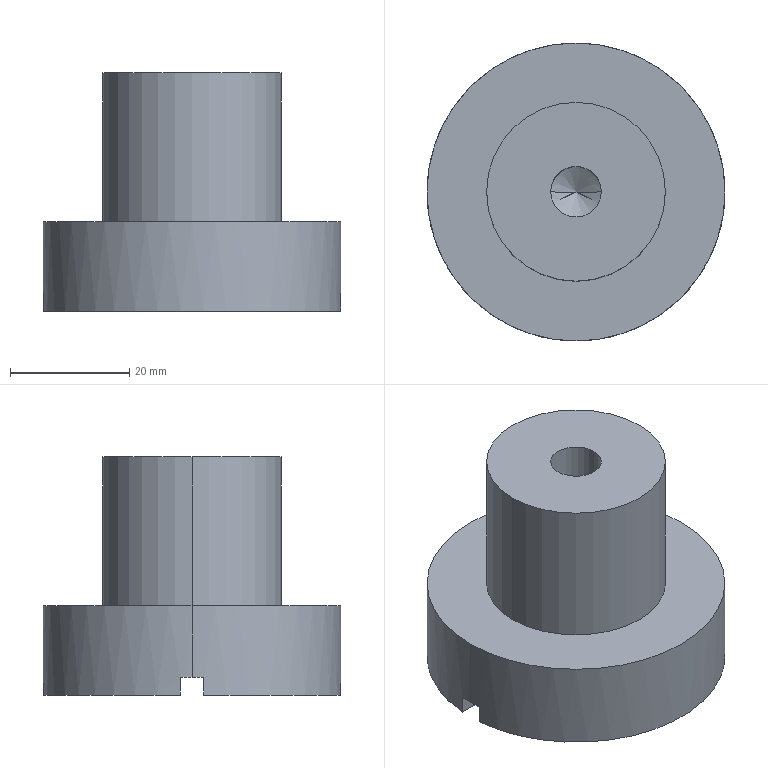Part | STEP file | Knob QY-1-20 | 1 solid | 15 faces | box 50 x 50 x 40 mm | volume 45086 mm3 | plane 7 | cylinder 6 | cone 2 | commonest cylinder face diameters 8.5 x2 30 x2 50 x2
STEP:
#1=CARTESIAN_POINT('',(0.,0.,0.));
#2=DIRECTION('',(0.,0.,1.));
#3=DIRECTION('',(1.,0.,0.));
#4=AXIS2_PLACEMENT_3D('',#1,#2,#3);
#5=CARTESIAN_POINT('',(4.25,0.,15.5));
#6=VERTEX_POINT('',#5);
#7=CARTESIAN_POINT('',(4.25,0.,40.));
#8=VERTEX_POINT('',#7);
#9=CARTESIAN_POINT('',(4.25,0.,40.));
#10=DIRECTION('',(0.,0.,1.));
#11=VECTOR('',#10,1.);
#12=LINE('',#9,#11);
#13=CARTESIAN_POINT('',(0.,0.,40.));
#14=DIRECTION('',(0.,0.,1.));
#15=DIRECTION('',(1.,0.,0.));
#16=AXIS2_PLACEMENT_3D('',#13,#14,#15);
#17=CYLINDRICAL_SURFACE('',#16,4.25);
#18=CARTESIAN_POINT('',(6.283,0.));
#19=DIRECTION('',(0.,1.));
#20=VECTOR('',#19,1.);
#21=LINE('',#18,#20);
#22=(GEOMETRIC_REPRESENTATION_CONTEXT(2)PARAMETRIC_REPRESENTATION_CONTEXT()REPRESENTATION_CONTEXT('',''));
#23=DEFINITIONAL_REPRESENTATION('',(#21),#22);
#24=PCURVE('',#17,#23);
#25=CARTESIAN_POINT('',(0.,0.,40.));
#26=DIRECTION('',(0.,0.,1.));
#27=DIRECTION('',(1.,0.,0.));
#28=AXIS2_PLACEMENT_3D('',#25,#26,#27);
#29=CYLINDRICAL_SURFACE('',#28,4.25);
#30=CARTESIAN_POINT('',(0.,0.));
#31=DIRECTION('',(0.,1.));
#32=VECTOR('',#31,1.);
#33=LINE('',#30,#32);
#34=(GEOMETRIC_REPRESENTATION_CONTEXT(2)PARAMETRIC_REPRESENTATION_CONTEXT()REPRESENTATION_CONTEXT('',''));
#35=DEFINITIONAL_REPRESENTATION('',(#33),#34);
#36=PCURVE('',#29,#35);
#37=SURFACE_CURVE('',#12,(#24,#36),.PCURVE_S1.);
#38=EDGE_CURVE('',#6,#8,#37,.T.);
#39=ORIENTED_EDGE('',*,*,#38,.T.);
#40=CARTESIAN_POINT('',(-4.25,0.,40.));
#41=VERTEX_POINT('',#40);
#42=CARTESIAN_POINT('',(0.,0.,40.));
#43=DIRECTION('',(0.,0.,1.));
#44=DIRECTION('',(1.,0.,0.));
#45=AXIS2_PLACEMENT_3D('',#42,#43,#44);
#46=CIRCLE('',#45,4.25);
#47=CARTESIAN_POINT('',(0.,0.));
#48=DIRECTION('',(1.,0.));
#49=VECTOR('',#48,1.);
#50=LINE('',#47,#49);
#51=(GEOMETRIC_REPRESENTATION_CONTEXT(2)PARAMETRIC_REPRESENTATION_CONTEXT()REPRESENTATION_CONTEXT('',''));
#52=DEFINITIONAL_REPRESENTATION('',(#50),#51);
#53=PCURVE('',#17,#52);
#54=CARTESIAN_POINT('',(0.,0.,40.));
#55=DIRECTION('',(0.,0.,1.));
#56=DIRECTION('',(1.,0.,0.));
#57=AXIS2_PLACEMENT_3D('',#54,#55,#56);
#58=PLANE('',#57);
#59=CARTESIAN_POINT('',(0.,0.));
#60=DIRECTION('',(1.,0.));
#61=AXIS2_PLACEMENT_2D('',#59,#60);
#62=CIRCLE('',#61,4.25);
#63=(GEOMETRIC_REPRESENTATION_CONTEXT(2)PARAMETRIC_REPRESENTATION_CONTEXT()REPRESENTATION_CONTEXT('',''));
#64=DEFINITIONAL_REPRESENTATION('',(#62),#63);
#65=PCURVE('',#58,#64);
#66=SURFACE_CURVE('',#46,(#53,#65),.PCURVE_S1.);
#67=EDGE_CURVE('',#41,#8,#66,.T.);
#68=ORIENTED_EDGE('',*,*,#67,.F.);
#69=CARTESIAN_POINT('',(-4.25,0.,15.5));
#70=VERTEX_POINT('',#69);
#71=CARTESIAN_POINT('',(-4.25,0.,40.));
#72=DIRECTION('',(0.,0.,1.));
#73=VECTOR('',#72,1.);
#74=LINE('',#71,#73);
#75=CARTESIAN_POINT('',(3.142,0.));
#76=DIRECTION('',(0.,1.));
#77=VECTOR('',#76,1.);
#78=LINE('',#75,#77);
#79=(GEOMETRIC_REPRESENTATION_CONTEXT(2)PARAMETRIC_REPRESENTATION_CONTEXT()REPRESENTATION_CONTEXT('',''));
#80=DEFINITIONAL_REPRESENTATION('',(#78),#79);
#81=PCURVE('',#17,#80);
#82=CARTESIAN_POINT('',(3.142,0.));
#83=DIRECTION('',(0.,1.));
#84=VECTOR('',#83,1.);
#85=LINE('',#82,#84);
#86=(GEOMETRIC_REPRESENTATION_CONTEXT(2)PARAMETRIC_REPRESENTATION_CONTEXT()REPRESENTATION_CONTEXT('',''));
#87=DEFINITIONAL_REPRESENTATION('',(#85),#86);
#88=PCURVE('',#29,#87);
#89=SURFACE_CURVE('',#74,(#81,#88),.PCURVE_S1.);
#90=EDGE_CURVE('',#70,#41,#89,.T.);
#91=ORIENTED_EDGE('',*,*,#90,.F.);
#92=CARTESIAN_POINT('',(0.,0.,15.5));
#93=DIRECTION('',(0.,0.,1.));
#94=DIRECTION('',(1.,0.,0.));
#95=AXIS2_PLACEMENT_3D('',#92,#93,#94);
#96=CIRCLE('',#95,4.25);
#97=CARTESIAN_POINT('',(0.,-24.5));
#98=DIRECTION('',(1.,0.));
#99=VECTOR('',#98,1.);
#100=LINE('',#97,#99);
#101=(GEOMETRIC_REPRESENTATION_CONTEXT(2)PARAMETRIC_REPRESENTATION_CONTEXT()REPRESENTATION_CONTEXT('',''));
#102=DEFINITIONAL_REPRESENTATION('',(#100),#101);
#103=PCURVE('',#17,#102);
#104=CARTESIAN_POINT('',(0.,0.,15.5));
#105=DIRECTION('',(0.,0.,1.));
#106=DIRECTION('',(1.,0.,0.));
#107=AXIS2_PLACEMENT_3D('',#104,#105,#106);
#108=CONICAL_SURFACE('',#107,4.25,1.03);
#109=CARTESIAN_POINT('',(0.,0.));
#110=DIRECTION('',(1.,0.));
#111=VECTOR('',#110,1.);
#112=LINE('',#109,#111);
#113=(GEOMETRIC_REPRESENTATION_CONTEXT(2)PARAMETRIC_REPRESENTATION_CONTEXT()REPRESENTATION_CONTEXT('',''));
#114=DEFINITIONAL_REPRESENTATION('',(#112),#113);
#115=PCURVE('',#108,#114);
#116=SURFACE_CURVE('',#96,(#103,#115),.PCURVE_S1.);
#117=EDGE_CURVE('',#70,#6,#116,.T.);
#118=ORIENTED_EDGE('',*,*,#117,.T.);
#119=EDGE_LOOP('',(#39,#68,#91,#118));
#120=FACE_BOUND('',#119,.F.);
#121=ADVANCED_FACE('',(#120),#17,.F.);
#122=ORIENTED_EDGE('',*,*,#117,.F.);
#123=CARTESIAN_POINT('',(0.,0.,12.946));
#124=VERTEX_POINT('',#123);
#125=CARTESIAN_POINT('',(-4.25,0.,15.5));
#126=DIRECTION('',(-0.8572,0.,0.515));
#127=VECTOR('',#126,1.);
#128=LINE('',#125,#127);
#129=CARTESIAN_POINT('',(3.142,0.));
#130=DIRECTION('',(0.,1.));
#131=VECTOR('',#130,1.);
#132=LINE('',#129,#131);
#133=(GEOMETRIC_REPRESENTATION_CONTEXT(2)PARAMETRIC_REPRESENTATION_CONTEXT()REPRESENTATION_CONTEXT('',''));
#134=DEFINITIONAL_REPRESENTATION('',(#132),#133);
#135=PCURVE('',#108,#134);
#136=CARTESIAN_POINT('',(0.,0.,15.5));
#137=DIRECTION('',(0.,0.,1.));
#138=DIRECTION('',(1.,0.,0.));
#139=AXIS2_PLACEMENT_3D('',#136,#137,#138);
#140=CONICAL_SURFACE('',#139,4.25,1.03);
#141=CARTESIAN_POINT('',(3.142,0.));
#142=DIRECTION('',(0.,1.));
#143=VECTOR('',#142,1.);
#144=LINE('',#141,#143);
#145=(GEOMETRIC_REPRESENTATION_CONTEXT(2)PARAMETRIC_REPRESENTATION_CONTEXT()REPRESENTATION_CONTEXT('',''));
#146=DEFINITIONAL_REPRESENTATION('',(#144),#145);
#147=PCURVE('',#140,#146);
#148=SURFACE_CURVE('',#128,(#135,#147),.PCURVE_S1.);
#149=EDGE_CURVE('',#124,#70,#148,.T.);
#150=ORIENTED_EDGE('',*,*,#149,.F.);
#151=CARTESIAN_POINT('',(4.25,0.,15.5));
#152=DIRECTION('',(0.8572,0.,0.515));
#153=VECTOR('',#152,1.);
#154=LINE('',#151,#153);
#155=CARTESIAN_POINT('',(6.283,0.));
#156=DIRECTION('',(0.,1.));
#157=VECTOR('',#156,1.);
#158=LINE('',#155,#157);
#159=(GEOMETRIC_REPRESENTATION_CONTEXT(2)PARAMETRIC_REPRESENTATION_CONTEXT()REPRESENTATION_CONTEXT('',''));
#160=DEFINITIONAL_REPRESENTATION('',(#158),#159);
#161=PCURVE('',#108,#160);
#162=CARTESIAN_POINT('',(0.,0.));
#163=DIRECTION('',(0.,1.));
#164=VECTOR('',#163,1.);
#165=LINE('',#162,#164);
#166=(GEOMETRIC_REPRESENTATION_CONTEXT(2)PARAMETRIC_REPRESENTATION_CONTEXT()REPRESENTATION_CONTEXT('',''));
#167=DEFINITIONAL_REPRESENTATION('',(#165),#166);
#168=PCURVE('',#140,#167);
#169=SURFACE_CURVE('',#154,(#161,#168),.PCURVE_S1.);
#170=EDGE_CURVE('',#124,#6,#169,.T.);
#171=ORIENTED_EDGE('',*,*,#170,.T.);
#172=EDGE_LOOP('',(#122,#150,#171));
#173=FACE_BOUND('',#172,.F.);
#174=ADVANCED_FACE('',(#173),#108,.F.);
#175=CARTESIAN_POINT('',(15.,0.,40.));
#176=VERTEX_POINT('',#175);
#177=CARTESIAN_POINT('',(-15.,0.,40.));
#178=VERTEX_POINT('',#177);
#179=CARTESIAN_POINT('',(0.,0.,40.));
#180=DIRECTION('',(0.,0.,1.));
#181=DIRECTION('',(1.,0.,0.));
#182=AXIS2_PLACEMENT_3D('',#179,#180,#181);
#183=CIRCLE('',#182,15.);
#184=CARTESIAN_POINT('',(0.,0.,40.));
#185=DIRECTION('',(0.,0.,-1.));
#186=DIRECTION('',(-1.,0.,0.));
#187=AXIS2_PLACEMENT_3D('',#184,#185,#186);
#188=CYLINDRICAL_SURFACE('',#187,15.);
#189=CARTESIAN_POINT('',(3.142,0.));
#190=DIRECTION('',(-1.,0.));
#191=VECTOR('',#190,1.);
#192=LINE('',#189,#191);
#193=(GEOMETRIC_REPRESENTATION_CONTEXT(2)PARAMETRIC_REPRESENTATION_CONTEXT()REPRESENTATION_CONTEXT('',''));
#194=DEFINITIONAL_REPRESENTATION('',(#192),#193);
#195=PCURVE('',#188,#194);
#196=CARTESIAN_POINT('',(0.,0.));
#197=DIRECTION('',(1.,0.));
#198=AXIS2_PLACEMENT_2D('',#196,#197);
#199=CIRCLE('',#198,15.);
#200=(GEOMETRIC_REPRESENTATION_CONTEXT(2)PARAMETRIC_REPRESENTATION_CONTEXT()REPRESENTATION_CONTEXT('',''));
#201=DEFINITIONAL_REPRESENTATION('',(#199),#200);
#202=PCURVE('',#58,#201);
#203=SURFACE_CURVE('',#183,(#195,#202),.PCURVE_S1.);
#204=EDGE_CURVE('',#176,#178,#203,.T.);
#205=ORIENTED_EDGE('',*,*,#204,.F.);
#206=CARTESIAN_POINT('',(15.,0.,15.));
#207=VERTEX_POINT('',#206);
#208=CARTESIAN_POINT('',(15.,0.,40.));
#209=DIRECTION('',(0.,0.,-1.));
#210=VECTOR('',#209,1.);
#211=LINE('',#208,#210);
#212=CARTESIAN_POINT('',(3.142,0.));
#213=DIRECTION('',(0.,1.));
#214=VECTOR('',#213,1.);
#215=LINE('',#212,#214);
#216=(GEOMETRIC_REPRESENTATION_CONTEXT(2)PARAMETRIC_REPRESENTATION_CONTEXT()REPRESENTATION_CONTEXT('',''));
#217=DEFINITIONAL_REPRESENTATION('',(#215),#216);
#218=PCURVE('',#188,#217);
#219=CARTESIAN_POINT('',(0.,0.,40.));
#220=DIRECTION('',(0.,0.,-1.));
#221=DIRECTION('',(-1.,0.,0.));
#222=AXIS2_PLACEMENT_3D('',#219,#220,#221);
#223=CYLINDRICAL_SURFACE('',#222,15.);
#224=CARTESIAN_POINT('',(3.142,0.));
#225=DIRECTION('',(0.,1.));
#226=VECTOR('',#225,1.);
#227=LINE('',#224,#226);
#228=(GEOMETRIC_REPRESENTATION_CONTEXT(2)PARAMETRIC_REPRESENTATION_CONTEXT()REPRESENTATION_CONTEXT('',''));
#229=DEFINITIONAL_REPRESENTATION('',(#227),#228);
#230=PCURVE('',#223,#229);
#231=SURFACE_CURVE('',#211,(#218,#230),.PCURVE_S1.);
#232=EDGE_CURVE('',#176,#207,#231,.T.);
#233=ORIENTED_EDGE('',*,*,#232,.T.);
#234=CARTESIAN_POINT('',(-15.,0.,15.));
#235=VERTEX_POINT('',#234);
#236=CARTESIAN_POINT('',(0.,0.,15.));
#237=DIRECTION('',(0.,0.,1.));
#238=DIRECTION('',(1.,0.,0.));
#239=AXIS2_PLACEMENT_3D('',#236,#237,#238);
#240=CIRCLE('',#239,15.);
#241=CARTESIAN_POINT('',(3.142,25.));
#242=DIRECTION('',(-1.,0.));
#243=VECTOR('',#242,1.);
#244=LINE('',#241,#243);
#245=(GEOMETRIC_REPRESENTATION_CONTEXT(2)PARAMETRIC_REPRESENTATION_CONTEXT()REPRESENTATION_CONTEXT('',''));
#246=DEFINITIONAL_REPRESENTATION('',(#244),#245);
#247=PCURVE('',#188,#246);
#248=CARTESIAN_POINT('',(0.,0.,15.));
#249=DIRECTION('',(0.,0.,1.));
#250=DIRECTION('',(1.,0.,0.));
#251=AXIS2_PLACEMENT_3D('',#248,#249,#250);
#252=PLANE('',#251);
#253=CARTESIAN_POINT('',(0.,0.));
#254=DIRECTION('',(1.,0.));
#255=AXIS2_PLACEMENT_2D('',#253,#254);
#256=CIRCLE('',#255,15.);
#257=(GEOMETRIC_REPRESENTATION_CONTEXT(2)PARAMETRIC_REPRESENTATION_CONTEXT()REPRESENTATION_CONTEXT('',''));
#258=DEFINITIONAL_REPRESENTATION('',(#256),#257);
#259=PCURVE('',#252,#258);
#260=SURFACE_CURVE('',#240,(#247,#259),.PCURVE_S1.);
#261=EDGE_CURVE('',#207,#235,#260,.T.);
#262=ORIENTED_EDGE('',*,*,#261,.T.);
#263=CARTESIAN_POINT('',(-15.,0.,40.));
#264=DIRECTION('',(0.,0.,-1.));
#265=VECTOR('',#264,1.);
#266=LINE('',#263,#265);
#267=CARTESIAN_POINT('',(0.,0.));
#268=DIRECTION('',(0.,1.));
#269=VECTOR('',#268,1.);
#270=LINE('',#267,#269);
#271=(GEOMETRIC_REPRESENTATION_CONTEXT(2)PARAMETRIC_REPRESENTATION_CONTEXT()REPRESENTATION_CONTEXT('',''));
#272=DEFINITIONAL_REPRESENTATION('',(#270),#271);
#273=PCURVE('',#188,#272);
#274=CARTESIAN_POINT('',(6.283,0.));
#275=DIRECTION('',(0.,1.));
#276=VECTOR('',#275,1.);
#277=LINE('',#274,#276);
#278=(GEOMETRIC_REPRESENTATION_CONTEXT(2)PARAMETRIC_REPRESENTATION_CONTEXT()REPRESENTATION_CONTEXT('',''));
#279=DEFINITIONAL_REPRESENTATION('',(#277),#278);
#280=PCURVE('',#223,#279);
#281=SURFACE_CURVE('',#266,(#273,#280),.PCURVE_S1.);
#282=EDGE_CURVE('',#178,#235,#281,.T.);
#283=ORIENTED_EDGE('',*,*,#282,.F.);
#284=EDGE_LOOP('',(#205,#233,#262,#283));
#285=FACE_BOUND('',#284,.T.);
#286=ADVANCED_FACE('',(#285),#188,.T.);
#287=CARTESIAN_POINT('',(25.,0.,15.));
#288=VERTEX_POINT('',#287);
#289=CARTESIAN_POINT('',(-25.,0.,15.));
#290=VERTEX_POINT('',#289);
#291=CARTESIAN_POINT('',(0.,0.,15.));
#292=DIRECTION('',(0.,0.,1.));
#293=DIRECTION('',(1.,0.,0.));
#294=AXIS2_PLACEMENT_3D('',#291,#292,#293);
#295=CIRCLE('',#294,25.);
#296=CARTESIAN_POINT('',(0.,0.,15.));
#297=DIRECTION('',(0.,0.,-1.));
#298=DIRECTION('',(-1.,0.,0.));
#299=AXIS2_PLACEMENT_3D('',#296,#297,#298);
#300=CYLINDRICAL_SURFACE('',#299,25.);
#301=CARTESIAN_POINT('',(3.142,0.));
#302=DIRECTION('',(-1.,0.));
#303=VECTOR('',#302,1.);
#304=LINE('',#301,#303);
#305=(GEOMETRIC_REPRESENTATION_CONTEXT(2)PARAMETRIC_REPRESENTATION_CONTEXT()REPRESENTATION_CONTEXT('',''));
#306=DEFINITIONAL_REPRESENTATION('',(#304),#305);
#307=PCURVE('',#300,#306);
#308=CARTESIAN_POINT('',(0.,0.));
#309=DIRECTION('',(1.,0.));
#310=AXIS2_PLACEMENT_2D('',#308,#309);
#311=CIRCLE('',#310,25.);
#312=(GEOMETRIC_REPRESENTATION_CONTEXT(2)PARAMETRIC_REPRESENTATION_CONTEXT()REPRESENTATION_CONTEXT('',''));
#313=DEFINITIONAL_REPRESENTATION('',(#311),#312);
#314=PCURVE('',#252,#313);
#315=SURFACE_CURVE('',#295,(#307,#314),.PCURVE_S1.);
#316=EDGE_CURVE('',#288,#290,#315,.T.);
#317=ORIENTED_EDGE('',*,*,#316,.F.);
#318=CARTESIAN_POINT('',(25.,0.,3.));
#319=VERTEX_POINT('',#318);
#320=CARTESIAN_POINT('',(25.,0.,15.));
#321=DIRECTION('',(0.,0.,-1.));
#322=VECTOR('',#321,1.);
#323=LINE('',#320,#322);
#324=CARTESIAN_POINT('',(3.142,0.));
#325=DIRECTION('',(0.,1.));
#326=VECTOR('',#325,1.);
#327=LINE('',#324,#326);
#328=(GEOMETRIC_REPRESENTATION_CONTEXT(2)PARAMETRIC_REPRESENTATION_CONTEXT()REPRESENTATION_CONTEXT('',''));
#329=DEFINITIONAL_REPRESENTATION('',(#327),#328);
#330=PCURVE('',#300,#329);
#331=CARTESIAN_POINT('',(0.,0.,15.));
#332=DIRECTION('',(0.,0.,-1.));
#333=DIRECTION('',(-1.,0.,0.));
#334=AXIS2_PLACEMENT_3D('',#331,#332,#333);
#335=CYLINDRICAL_SURFACE('',#334,25.);
#336=CARTESIAN_POINT('',(3.142,0.));
#337=DIRECTION('',(0.,1.));
#338=VECTOR('',#337,1.);
#339=LINE('',#336,#338);
#340=(GEOMETRIC_REPRESENTATION_CONTEXT(2)PARAMETRIC_REPRESENTATION_CONTEXT()REPRESENTATION_CONTEXT('',''));
#341=DEFINITIONAL_REPRESENTATION('',(#339),#340);
#342=PCURVE('',#335,#341);
#343=SURFACE_CURVE('',#323,(#330,#342),.PCURVE_S1.);
#344=EDGE_CURVE('',#288,#319,#343,.T.);
#345=ORIENTED_EDGE('',*,*,#344,.T.);
#346=CARTESIAN_POINT('',(24.92,2.,3.));
#347=VERTEX_POINT('',#346);
#348=CARTESIAN_POINT('',(0.,0.,3.));
#349=DIRECTION('',(0.,0.,-1.));
#350=DIRECTION('',(-1.,0.,0.));
#351=AXIS2_PLACEMENT_3D('',#348,#349,#350);
#352=CIRCLE('',#351,25.);
#353=CARTESIAN_POINT('',(0.,12.));
#354=DIRECTION('',(1.,0.));
#355=VECTOR('',#354,1.);
#356=LINE('',#353,#355);
#357=(GEOMETRIC_REPRESENTATION_CONTEXT(2)PARAMETRIC_REPRESENTATION_CONTEXT()REPRESENTATION_CONTEXT('',''));
#358=DEFINITIONAL_REPRESENTATION('',(#356),#357);
#359=PCURVE('',#300,#358);
#360=CARTESIAN_POINT('',(0.,0.,3.));
#361=DIRECTION('',(0.,0.,-1.));
#362=DIRECTION('',(-1.,0.,0.));
#363=AXIS2_PLACEMENT_3D('',#360,#361,#362);
#364=PLANE('',#363);
#365=CARTESIAN_POINT('',(0.,0.));
#366=DIRECTION('',(1.,0.));
#367=AXIS2_PLACEMENT_2D('',#365,#366);
#368=CIRCLE('',#367,25.);
#369=(GEOMETRIC_REPRESENTATION_CONTEXT(2)PARAMETRIC_REPRESENTATION_CONTEXT()REPRESENTATION_CONTEXT('',''));
#370=DEFINITIONAL_REPRESENTATION('',(#368),#369);
#371=PCURVE('',#364,#370);
#372=SURFACE_CURVE('',#352,(#359,#371),.PCURVE_S1.);
#373=EDGE_CURVE('',#347,#319,#372,.T.);
#374=ORIENTED_EDGE('',*,*,#373,.F.);
#375=CARTESIAN_POINT('',(24.92,2.,0.));
#376=VERTEX_POINT('',#375);
#377=CARTESIAN_POINT('',(24.92,2.,15.));
#378=DIRECTION('',(0.,0.,-1.));
#379=VECTOR('',#378,1.);
#380=LINE('',#377,#379);
#381=CARTESIAN_POINT('',(3.062,0.));
#382=DIRECTION('',(0.,1.));
#383=VECTOR('',#382,1.);
#384=LINE('',#381,#383);
#385=(GEOMETRIC_REPRESENTATION_CONTEXT(2)PARAMETRIC_REPRESENTATION_CONTEXT()REPRESENTATION_CONTEXT('',''));
#386=DEFINITIONAL_REPRESENTATION('',(#384),#385);
#387=PCURVE('',#300,#386);
#388=CARTESIAN_POINT('',(34.879,2.,3.));
#389=DIRECTION('',(0.,1.,0.));
#390=DIRECTION('',(0.,0.,1.));
#391=AXIS2_PLACEMENT_3D('',#388,#389,#390);
#392=PLANE('',#391);
#393=CARTESIAN_POINT('',(12.,-9.959));
#394=DIRECTION('',(-1.,0.));
#395=VECTOR('',#394,1.);
#396=LINE('',#393,#395);
#397=(GEOMETRIC_REPRESENTATION_CONTEXT(2)PARAMETRIC_REPRESENTATION_CONTEXT()REPRESENTATION_CONTEXT('',''));
#398=DEFINITIONAL_REPRESENTATION('',(#396),#397);
#399=PCURVE('',#392,#398);
#400=SURFACE_CURVE('',#380,(#387,#399),.PCURVE_S1.);
#401=EDGE_CURVE('',#347,#376,#400,.T.);
#402=ORIENTED_EDGE('',*,*,#401,.T.);
#403=CARTESIAN_POINT('',(-24.92,2.,0.));
#404=VERTEX_POINT('',#403);
#405=CARTESIAN_POINT('',(0.,0.,0.));
#406=DIRECTION('',(0.,0.,1.));
#407=DIRECTION('',(1.,0.,0.));
#408=AXIS2_PLACEMENT_3D('',#405,#406,#407);
#409=CIRCLE('',#408,25.);
#410=CARTESIAN_POINT('',(3.142,15.));
#411=DIRECTION('',(-1.,0.));
#412=VECTOR('',#411,1.);
#413=LINE('',#410,#412);
#414=(GEOMETRIC_REPRESENTATION_CONTEXT(2)PARAMETRIC_REPRESENTATION_CONTEXT()REPRESENTATION_CONTEXT('',''));
#415=DEFINITIONAL_REPRESENTATION('',(#413),#414);
#416=PCURVE('',#300,#415);
#417=CARTESIAN_POINT('',(0.,0.,0.));
#418=DIRECTION('',(0.,0.,1.));
#419=DIRECTION('',(1.,0.,0.));
#420=AXIS2_PLACEMENT_3D('',#417,#418,#419);
#421=PLANE('',#420);
#422=CARTESIAN_POINT('',(0.,0.));
#423=DIRECTION('',(1.,0.));
#424=AXIS2_PLACEMENT_2D('',#422,#423);
#425=CIRCLE('',#424,25.);
#426=(GEOMETRIC_REPRESENTATION_CONTEXT(2)PARAMETRIC_REPRESENTATION_CONTEXT()REPRESENTATION_CONTEXT('',''));
#427=DEFINITIONAL_REPRESENTATION('',(#425),#426);
#428=PCURVE('',#421,#427);
#429=SURFACE_CURVE('',#409,(#416,#428),.PCURVE_S1.);
#430=EDGE_CURVE('',#376,#404,#429,.T.);
#431=ORIENTED_EDGE('',*,*,#430,.T.);
#432=CARTESIAN_POINT('',(-24.92,2.,3.));
#433=VERTEX_POINT('',#432);
#434=CARTESIAN_POINT('',(-24.92,2.,15.));
#435=DIRECTION('',(0.,0.,1.));
#436=VECTOR('',#435,1.);
#437=LINE('',#434,#436);
#438=CARTESIAN_POINT('',(0.08009,0.));
#439=DIRECTION('',(0.,-1.));
#440=VECTOR('',#439,1.);
#441=LINE('',#438,#440);
#442=(GEOMETRIC_REPRESENTATION_CONTEXT(2)PARAMETRIC_REPRESENTATION_CONTEXT()REPRESENTATION_CONTEXT('',''));
#443=DEFINITIONAL_REPRESENTATION('',(#441),#442);
#444=PCURVE('',#300,#443);
#445=CARTESIAN_POINT('',(12.,-59.799));
#446=DIRECTION('',(1.,0.));
#447=VECTOR('',#446,1.);
#448=LINE('',#445,#447);
#449=(GEOMETRIC_REPRESENTATION_CONTEXT(2)PARAMETRIC_REPRESENTATION_CONTEXT()REPRESENTATION_CONTEXT('',''));
#450=DEFINITIONAL_REPRESENTATION('',(#448),#449);
#451=PCURVE('',#392,#450);
#452=SURFACE_CURVE('',#437,(#444,#451),.PCURVE_S1.);
#453=EDGE_CURVE('',#404,#433,#452,.T.);
#454=ORIENTED_EDGE('',*,*,#453,.T.);
#455=CARTESIAN_POINT('',(-25.,0.,3.));
#456=VERTEX_POINT('',#455);
#457=CARTESIAN_POINT('',(0.,0.,3.));
#458=DIRECTION('',(0.,0.,-1.));
#459=DIRECTION('',(-1.,0.,0.));
#460=AXIS2_PLACEMENT_3D('',#457,#458,#459);
#461=CIRCLE('',#460,25.);
#462=CARTESIAN_POINT('',(0.,12.));
#463=DIRECTION('',(1.,0.));
#464=VECTOR('',#463,1.);
#465=LINE('',#462,#464);
#466=(GEOMETRIC_REPRESENTATION_CONTEXT(2)PARAMETRIC_REPRESENTATION_CONTEXT()REPRESENTATION_CONTEXT('',''));
#467=DEFINITIONAL_REPRESENTATION('',(#465),#466);
#468=PCURVE('',#300,#467);
#469=CARTESIAN_POINT('',(0.,0.));
#470=DIRECTION('',(1.,0.));
#471=AXIS2_PLACEMENT_2D('',#469,#470);
#472=CIRCLE('',#471,25.);
#473=(GEOMETRIC_REPRESENTATION_CONTEXT(2)PARAMETRIC_REPRESENTATION_CONTEXT()REPRESENTATION_CONTEXT('',''));
#474=DEFINITIONAL_REPRESENTATION('',(#472),#473);
#475=PCURVE('',#364,#474);
#476=SURFACE_CURVE('',#461,(#468,#475),.PCURVE_S1.);
#477=EDGE_CURVE('',#456,#433,#476,.T.);
#478=ORIENTED_EDGE('',*,*,#477,.F.);
#479=CARTESIAN_POINT('',(-25.,0.,15.));
#480=DIRECTION('',(0.,0.,-1.));
#481=VECTOR('',#480,1.);
#482=LINE('',#479,#481);
#483=CARTESIAN_POINT('',(0.,0.));
#484=DIRECTION('',(0.,1.));
#485=VECTOR('',#484,1.);
#486=LINE('',#483,#485);
#487=(GEOMETRIC_REPRESENTATION_CONTEXT(2)PARAMETRIC_REPRESENTATION_CONTEXT()REPRESENTATION_CONTEXT('',''));
#488=DEFINITIONAL_REPRESENTATION('',(#486),#487);
#489=PCURVE('',#300,#488);
#490=CARTESIAN_POINT('',(6.283,0.));
#491=DIRECTION('',(0.,1.));
#492=VECTOR('',#491,1.);
#493=LINE('',#490,#492);
#494=(GEOMETRIC_REPRESENTATION_CONTEXT(2)PARAMETRIC_REPRESENTATION_CONTEXT()REPRESENTATION_CONTEXT('',''));
#495=DEFINITIONAL_REPRESENTATION('',(#493),#494);
#496=PCURVE('',#335,#495);
#497=SURFACE_CURVE('',#482,(#489,#496),.PCURVE_S1.);
#498=EDGE_CURVE('',#290,#456,#497,.T.);
#499=ORIENTED_EDGE('',*,*,#498,.F.);
#500=EDGE_LOOP('',(#317,#345,#374,#402,#431,#454,#478,#499));
#501=FACE_BOUND('',#500,.T.);
#502=ADVANCED_FACE('',(#501),#300,.T.);
#503=CARTESIAN_POINT('',(-24.92,-2.,0.));
#504=VERTEX_POINT('',#503);
#505=CARTESIAN_POINT('',(24.92,-2.,0.));
#506=VERTEX_POINT('',#505);
#507=CARTESIAN_POINT('',(0.,0.,0.));
#508=DIRECTION('',(0.,0.,1.));
#509=DIRECTION('',(1.,0.,0.));
#510=AXIS2_PLACEMENT_3D('',#507,#508,#509);
#511=CIRCLE('',#510,25.);
#512=CARTESIAN_POINT('',(0.,0.,0.));
#513=DIRECTION('',(0.,0.,1.));
#514=DIRECTION('',(1.,0.,0.));
#515=AXIS2_PLACEMENT_3D('',#512,#513,#514);
#516=PLANE('',#515);
#517=CARTESIAN_POINT('',(0.,0.));
#518=DIRECTION('',(1.,0.));
#519=AXIS2_PLACEMENT_2D('',#517,#518);
#520=CIRCLE('',#519,25.);
#521=(GEOMETRIC_REPRESENTATION_CONTEXT(2)PARAMETRIC_REPRESENTATION_CONTEXT()REPRESENTATION_CONTEXT('',''));
#522=DEFINITIONAL_REPRESENTATION('',(#520),#521);
#523=PCURVE('',#516,#522);
#524=CARTESIAN_POINT('',(9.425,15.));
#525=DIRECTION('',(-1.,0.));
#526=VECTOR('',#525,1.);
#527=LINE('',#524,#526);
#528=(GEOMETRIC_REPRESENTATION_CONTEXT(2)PARAMETRIC_REPRESENTATION_CONTEXT()REPRESENTATION_CONTEXT('',''));
#529=DEFINITIONAL_REPRESENTATION('',(#527),#528);
#530=PCURVE('',#335,#529);
#531=SURFACE_CURVE('',#511,(#523,#530),.PCURVE_S1.);
#532=EDGE_CURVE('',#504,#506,#531,.T.);
#533=ORIENTED_EDGE('',*,*,#532,.F.);
#534=CARTESIAN_POINT('',(0.,-2.,0.));
#535=DIRECTION('',(1.,0.,0.));
#536=VECTOR('',#535,1.);
#537=LINE('',#534,#536);
#538=CARTESIAN_POINT('',(0.,-2.));
#539=DIRECTION('',(1.,0.));
#540=VECTOR('',#539,1.);
#541=LINE('',#538,#540);
#542=(GEOMETRIC_REPRESENTATION_CONTEXT(2)PARAMETRIC_REPRESENTATION_CONTEXT()REPRESENTATION_CONTEXT('',''));
#543=DEFINITIONAL_REPRESENTATION('',(#541),#542);
#544=PCURVE('',#516,#543);
#545=CARTESIAN_POINT('',(34.879,-2.,3.));
#546=DIRECTION('',(0.,-1.,0.));
#547=DIRECTION('',(0.,0.,-1.));
#548=AXIS2_PLACEMENT_3D('',#545,#546,#547);
#549=PLANE('',#548);
#550=CARTESIAN_POINT('',(3.,-34.879));
#551=DIRECTION('',(0.,1.));
#552=VECTOR('',#551,1.);
#553=LINE('',#550,#552);
#554=(GEOMETRIC_REPRESENTATION_CONTEXT(2)PARAMETRIC_REPRESENTATION_CONTEXT()REPRESENTATION_CONTEXT('',''));
#555=DEFINITIONAL_REPRESENTATION('',(#553),#554);
#556=PCURVE('',#549,#555);
#557=SURFACE_CURVE('',#537,(#544,#556),.PCURVE_S1.);
#558=EDGE_CURVE('',#504,#506,#557,.T.);
#559=ORIENTED_EDGE('',*,*,#558,.T.);
#560=EDGE_LOOP('',(#533,#559));
#561=FACE_BOUND('',#560,.T.);
#562=ADVANCED_FACE('',(#561),#516,.F.);
#563=ORIENTED_EDGE('',*,*,#344,.F.);
#564=CARTESIAN_POINT('',(0.,0.,15.));
#565=DIRECTION('',(0.,0.,1.));
#566=DIRECTION('',(1.,0.,0.));
#567=AXIS2_PLACEMENT_3D('',#564,#565,#566);
#568=CIRCLE('',#567,25.);
#569=CARTESIAN_POINT('',(9.425,0.));
#570=DIRECTION('',(-1.,0.));
#571=VECTOR('',#570,1.);
#572=LINE('',#569,#571);
#573=(GEOMETRIC_REPRESENTATION_CONTEXT(2)PARAMETRIC_REPRESENTATION_CONTEXT()REPRESENTATION_CONTEXT('',''));
#574=DEFINITIONAL_REPRESENTATION('',(#572),#573);
#575=PCURVE('',#335,#574);
#576=CARTESIAN_POINT('',(0.,0.));
#577=DIRECTION('',(1.,0.));
#578=AXIS2_PLACEMENT_2D('',#576,#577);
#579=CIRCLE('',#578,25.);
#580=(GEOMETRIC_REPRESENTATION_CONTEXT(2)PARAMETRIC_REPRESENTATION_CONTEXT()REPRESENTATION_CONTEXT('',''));
#581=DEFINITIONAL_REPRESENTATION('',(#579),#580);
#582=PCURVE('',#252,#581);
#583=SURFACE_CURVE('',#568,(#575,#582),.PCURVE_S1.);
#584=EDGE_CURVE('',#290,#288,#583,.T.);
#585=ORIENTED_EDGE('',*,*,#584,.F.);
#586=ORIENTED_EDGE('',*,*,#498,.T.);
#587=CARTESIAN_POINT('',(-24.92,-2.,3.));
#588=VERTEX_POINT('',#587);
#589=CARTESIAN_POINT('',(0.,0.,3.));
#590=DIRECTION('',(0.,0.,-1.));
#591=DIRECTION('',(-1.,0.,0.));
#592=AXIS2_PLACEMENT_3D('',#589,#590,#591);
#593=CIRCLE('',#592,25.);
#594=CARTESIAN_POINT('',(0.,12.));
#595=DIRECTION('',(1.,0.));
#596=VECTOR('',#595,1.);
#597=LINE('',#594,#596);
#598=(GEOMETRIC_REPRESENTATION_CONTEXT(2)PARAMETRIC_REPRESENTATION_CONTEXT()REPRESENTATION_CONTEXT('',''));
#599=DEFINITIONAL_REPRESENTATION('',(#597),#598);
#600=PCURVE('',#335,#599);
#601=CARTESIAN_POINT('',(0.,0.));
#602=DIRECTION('',(1.,0.));
#603=AXIS2_PLACEMENT_2D('',#601,#602);
#604=CIRCLE('',#603,25.);
#605=(GEOMETRIC_REPRESENTATION_CONTEXT(2)PARAMETRIC_REPRESENTATION_CONTEXT()REPRESENTATION_CONTEXT('',''));
#606=DEFINITIONAL_REPRESENTATION('',(#604),#605);
#607=PCURVE('',#364,#606);
#608=SURFACE_CURVE('',#593,(#600,#607),.PCURVE_S1.);
#609=EDGE_CURVE('',#588,#456,#608,.T.);
#610=ORIENTED_EDGE('',*,*,#609,.F.);
#611=CARTESIAN_POINT('',(-24.92,-2.,15.));
#612=DIRECTION('',(0.,0.,-1.));
#613=VECTOR('',#612,1.);
#614=LINE('',#611,#613);
#615=CARTESIAN_POINT('',(6.203,0.));
#616=DIRECTION('',(0.,1.));
#617=VECTOR('',#616,1.);
#618=LINE('',#615,#617);
#619=(GEOMETRIC_REPRESENTATION_CONTEXT(2)PARAMETRIC_REPRESENTATION_CONTEXT()REPRESENTATION_CONTEXT('',''));
#620=DEFINITIONAL_REPRESENTATION('',(#618),#619);
#621=PCURVE('',#335,#620);
#622=CARTESIAN_POINT('',(-12.,-59.799));
#623=DIRECTION('',(1.,0.));
#624=VECTOR('',#623,1.);
#625=LINE('',#622,#624);
#626=(GEOMETRIC_REPRESENTATION_CONTEXT(2)PARAMETRIC_REPRESENTATION_CONTEXT()REPRESENTATION_CONTEXT('',''));
#627=DEFINITIONAL_REPRESENTATION('',(#625),#626);
#628=PCURVE('',#549,#627);
#629=SURFACE_CURVE('',#614,(#621,#628),.PCURVE_S1.);
#630=EDGE_CURVE('',#588,#504,#629,.T.);
#631=ORIENTED_EDGE('',*,*,#630,.T.);
#632=ORIENTED_EDGE('',*,*,#532,.T.);
#633=CARTESIAN_POINT('',(24.92,-2.,3.));
#634=VERTEX_POINT('',#633);
#635=CARTESIAN_POINT('',(24.92,-2.,15.));
#636=DIRECTION('',(0.,0.,1.));
#637=VECTOR('',#636,1.);
#638=LINE('',#635,#637);
#639=CARTESIAN_POINT('',(3.222,0.));
#640=DIRECTION('',(0.,-1.));
#641=VECTOR('',#640,1.);
#642=LINE('',#639,#641);
#643=(GEOMETRIC_REPRESENTATION_CONTEXT(2)PARAMETRIC_REPRESENTATION_CONTEXT()REPRESENTATION_CONTEXT('',''));
#644=DEFINITIONAL_REPRESENTATION('',(#642),#643);
#645=PCURVE('',#335,#644);
#646=CARTESIAN_POINT('',(-12.,-9.959));
#647=DIRECTION('',(-1.,0.));
#648=VECTOR('',#647,1.);
#649=LINE('',#646,#648);
#650=(GEOMETRIC_REPRESENTATION_CONTEXT(2)PARAMETRIC_REPRESENTATION_CONTEXT()REPRESENTATION_CONTEXT('',''));
#651=DEFINITIONAL_REPRESENTATION('',(#649),#650);
#652=PCURVE('',#549,#651);
#653=SURFACE_CURVE('',#638,(#645,#652),.PCURVE_S1.);
#654=EDGE_CURVE('',#506,#634,#653,.T.);
#655=ORIENTED_EDGE('',*,*,#654,.T.);
#656=CARTESIAN_POINT('',(0.,0.,3.));
#657=DIRECTION('',(0.,0.,-1.));
#658=DIRECTION('',(-1.,0.,0.));
#659=AXIS2_PLACEMENT_3D('',#656,#657,#658);
#660=CIRCLE('',#659,25.);
#661=CARTESIAN_POINT('',(0.,12.));
#662=DIRECTION('',(1.,0.));
#663=VECTOR('',#662,1.);
#664=LINE('',#661,#663);
#665=(GEOMETRIC_REPRESENTATION_CONTEXT(2)PARAMETRIC_REPRESENTATION_CONTEXT()REPRESENTATION_CONTEXT('',''));
#666=DEFINITIONAL_REPRESENTATION('',(#664),#665);
#667=PCURVE('',#335,#666);
#668=CARTESIAN_POINT('',(0.,0.));
#669=DIRECTION('',(1.,0.));
#670=AXIS2_PLACEMENT_2D('',#668,#669);
#671=CIRCLE('',#670,25.);
#672=(GEOMETRIC_REPRESENTATION_CONTEXT(2)PARAMETRIC_REPRESENTATION_CONTEXT()REPRESENTATION_CONTEXT('',''));
#673=DEFINITIONAL_REPRESENTATION('',(#671),#672);
#674=PCURVE('',#364,#673);
#675=SURFACE_CURVE('',#660,(#667,#674),.PCURVE_S1.);
#676=EDGE_CURVE('',#319,#634,#675,.T.);
#677=ORIENTED_EDGE('',*,*,#676,.F.);
#678=EDGE_LOOP('',(#563,#585,#586,#610,#631,#632,#655,#677));
#679=FACE_BOUND('',#678,.T.);
#680=ADVANCED_FACE('',(#679),#335,.T.);
#681=CARTESIAN_POINT('',(0.,0.,15.));
#682=DIRECTION('',(0.,0.,1.));
#683=DIRECTION('',(1.,0.,0.));
#684=AXIS2_PLACEMENT_3D('',#681,#682,#683);
#685=CIRCLE('',#684,15.);
#686=CARTESIAN_POINT('',(0.,0.));
#687=DIRECTION('',(1.,0.));
#688=AXIS2_PLACEMENT_2D('',#686,#687);
#689=CIRCLE('',#688,15.);
#690=(GEOMETRIC_REPRESENTATION_CONTEXT(2)PARAMETRIC_REPRESENTATION_CONTEXT()REPRESENTATION_CONTEXT('',''));
#691=DEFINITIONAL_REPRESENTATION('',(#689),#690);
#692=PCURVE('',#252,#691);
#693=CARTESIAN_POINT('',(9.425,25.));
#694=DIRECTION('',(-1.,0.));
#695=VECTOR('',#694,1.);
#696=LINE('',#693,#695);
#697=(GEOMETRIC_REPRESENTATION_CONTEXT(2)PARAMETRIC_REPRESENTATION_CONTEXT()REPRESENTATION_CONTEXT('',''));
#698=DEFINITIONAL_REPRESENTATION('',(#696),#697);
#699=PCURVE('',#223,#698);
#700=SURFACE_CURVE('',#685,(#692,#699),.PCURVE_S1.);
#701=EDGE_CURVE('',#235,#207,#700,.T.);
#702=ORIENTED_EDGE('',*,*,#701,.F.);
#703=ORIENTED_EDGE('',*,*,#261,.F.);
#704=EDGE_LOOP('',(#702,#703));
#705=FACE_BOUND('',#704,.T.);
#706=ORIENTED_EDGE('',*,*,#584,.T.);
#707=ORIENTED_EDGE('',*,*,#316,.T.);
#708=EDGE_LOOP('',(#706,#707));
#709=FACE_BOUND('',#708,.T.);
#710=ADVANCED_FACE('',(#705,#709),#252,.T.);
#711=ORIENTED_EDGE('',*,*,#430,.F.);
#712=CARTESIAN_POINT('',(0.,2.,0.));
#713=DIRECTION('',(-1.,0.,0.));
#714=VECTOR('',#713,1.);
#715=LINE('',#712,#714);
#716=CARTESIAN_POINT('',(0.,2.));
#717=DIRECTION('',(-1.,0.));
#718=VECTOR('',#717,1.);
#719=LINE('',#716,#718);
#720=(GEOMETRIC_REPRESENTATION_CONTEXT(2)PARAMETRIC_REPRESENTATION_CONTEXT()REPRESENTATION_CONTEXT('',''));
#721=DEFINITIONAL_REPRESENTATION('',(#719),#720);
#722=PCURVE('',#421,#721);
#723=CARTESIAN_POINT('',(-3.,-34.879));
#724=DIRECTION('',(0.,-1.));
#725=VECTOR('',#724,1.);
#726=LINE('',#723,#725);
#727=(GEOMETRIC_REPRESENTATION_CONTEXT(2)PARAMETRIC_REPRESENTATION_CONTEXT()REPRESENTATION_CONTEXT('',''));
#728=DEFINITIONAL_REPRESENTATION('',(#726),#727);
#729=PCURVE('',#392,#728);
#730=SURFACE_CURVE('',#715,(#722,#729),.PCURVE_S1.);
#731=EDGE_CURVE('',#376,#404,#730,.T.);
#732=ORIENTED_EDGE('',*,*,#731,.T.);
#733=EDGE_LOOP('',(#711,#732));
#734=FACE_BOUND('',#733,.T.);
#735=ADVANCED_FACE('',(#734),#421,.F.);
#736=ORIENTED_EDGE('',*,*,#232,.F.);
#737=CARTESIAN_POINT('',(0.,0.,40.));
#738=DIRECTION('',(0.,0.,1.));
#739=DIRECTION('',(1.,0.,0.));
#740=AXIS2_PLACEMENT_3D('',#737,#738,#739);
#741=CIRCLE('',#740,15.);
#742=CARTESIAN_POINT('',(9.425,0.));
#743=DIRECTION('',(-1.,0.));
#744=VECTOR('',#743,1.);
#745=LINE('',#742,#744);
#746=(GEOMETRIC_REPRESENTATION_CONTEXT(2)PARAMETRIC_REPRESENTATION_CONTEXT()REPRESENTATION_CONTEXT('',''));
#747=DEFINITIONAL_REPRESENTATION('',(#745),#746);
#748=PCURVE('',#223,#747);
#749=CARTESIAN_POINT('',(0.,0.));
#750=DIRECTION('',(1.,0.));
#751=AXIS2_PLACEMENT_2D('',#749,#750);
#752=CIRCLE('',#751,15.);
#753=(GEOMETRIC_REPRESENTATION_CONTEXT(2)PARAMETRIC_REPRESENTATION_CONTEXT()REPRESENTATION_CONTEXT('',''));
#754=DEFINITIONAL_REPRESENTATION('',(#752),#753);
#755=PCURVE('',#58,#754);
#756=SURFACE_CURVE('',#741,(#748,#755),.PCURVE_S1.);
#757=EDGE_CURVE('',#178,#176,#756,.T.);
#758=ORIENTED_EDGE('',*,*,#757,.F.);
#759=ORIENTED_EDGE('',*,*,#282,.T.);
#760=ORIENTED_EDGE('',*,*,#701,.T.);
#761=EDGE_LOOP('',(#736,#758,#759,#760));
#762=FACE_BOUND('',#761,.T.);
#763=ADVANCED_FACE('',(#762),#223,.T.);
#764=CARTESIAN_POINT('',(0.,0.,40.));
#765=DIRECTION('',(0.,0.,1.));
#766=DIRECTION('',(1.,0.,0.));
#767=AXIS2_PLACEMENT_3D('',#764,#765,#766);
#768=CIRCLE('',#767,4.25);
#769=CARTESIAN_POINT('',(0.,0.));
#770=DIRECTION('',(1.,0.));
#771=AXIS2_PLACEMENT_2D('',#769,#770);
#772=CIRCLE('',#771,4.25);
#773=(GEOMETRIC_REPRESENTATION_CONTEXT(2)PARAMETRIC_REPRESENTATION_CONTEXT()REPRESENTATION_CONTEXT('',''));
#774=DEFINITIONAL_REPRESENTATION('',(#772),#773);
#775=PCURVE('',#58,#774);
#776=CARTESIAN_POINT('',(0.,0.));
#777=DIRECTION('',(1.,0.));
#778=VECTOR('',#777,1.);
#779=LINE('',#776,#778);
#780=(GEOMETRIC_REPRESENTATION_CONTEXT(2)PARAMETRIC_REPRESENTATION_CONTEXT()REPRESENTATION_CONTEXT('',''));
#781=DEFINITIONAL_REPRESENTATION('',(#779),#780);
#782=PCURVE('',#29,#781);
#783=SURFACE_CURVE('',#768,(#775,#782),.PCURVE_S1.);
#784=EDGE_CURVE('',#8,#41,#783,.T.);
#785=ORIENTED_EDGE('',*,*,#784,.F.);
#786=ORIENTED_EDGE('',*,*,#67,.F.);
#787=EDGE_LOOP('',(#785,#786));
#788=FACE_BOUND('',#787,.T.);
#789=ORIENTED_EDGE('',*,*,#757,.T.);
#790=ORIENTED_EDGE('',*,*,#204,.T.);
#791=EDGE_LOOP('',(#789,#790));
#792=FACE_BOUND('',#791,.T.);
#793=ADVANCED_FACE('',(#788,#792),#58,.T.);
#794=ORIENTED_EDGE('',*,*,#373,.T.);
#795=ORIENTED_EDGE('',*,*,#676,.T.);
#796=CARTESIAN_POINT('',(34.879,-2.,3.));
#797=DIRECTION('',(-1.,0.,0.));
#798=VECTOR('',#797,1.);
#799=LINE('',#796,#798);
#800=CARTESIAN_POINT('',(-34.879,-2.));
#801=DIRECTION('',(1.,0.));
#802=VECTOR('',#801,1.);
#803=LINE('',#800,#802);
#804=(GEOMETRIC_REPRESENTATION_CONTEXT(2)PARAMETRIC_REPRESENTATION_CONTEXT()REPRESENTATION_CONTEXT('',''));
#805=DEFINITIONAL_REPRESENTATION('',(#803),#804);
#806=PCURVE('',#364,#805);
#807=CARTESIAN_POINT('',(0.,0.));
#808=DIRECTION('',(0.,-1.));
#809=VECTOR('',#808,1.);
#810=LINE('',#807,#809);
#811=(GEOMETRIC_REPRESENTATION_CONTEXT(2)PARAMETRIC_REPRESENTATION_CONTEXT()REPRESENTATION_CONTEXT('',''));
#812=DEFINITIONAL_REPRESENTATION('',(#810),#811);
#813=PCURVE('',#549,#812);
#814=SURFACE_CURVE('',#799,(#806,#813),.PCURVE_S1.);
#815=EDGE_CURVE('',#634,#588,#814,.T.);
#816=ORIENTED_EDGE('',*,*,#815,.T.);
#817=ORIENTED_EDGE('',*,*,#609,.T.);
#818=ORIENTED_EDGE('',*,*,#477,.T.);
#819=CARTESIAN_POINT('',(34.879,2.,3.));
#820=DIRECTION('',(1.,0.,0.));
#821=VECTOR('',#820,1.);
#822=LINE('',#819,#821);
#823=CARTESIAN_POINT('',(-34.879,2.));
#824=DIRECTION('',(-1.,0.));
#825=VECTOR('',#824,1.);
#826=LINE('',#823,#825);
#827=(GEOMETRIC_REPRESENTATION_CONTEXT(2)PARAMETRIC_REPRESENTATION_CONTEXT()REPRESENTATION_CONTEXT('',''));
#828=DEFINITIONAL_REPRESENTATION('',(#826),#827);
#829=PCURVE('',#364,#828);
#830=CARTESIAN_POINT('',(0.,0.));
#831=DIRECTION('',(0.,1.));
#832=VECTOR('',#831,1.);
#833=LINE('',#830,#832);
#834=(GEOMETRIC_REPRESENTATION_CONTEXT(2)PARAMETRIC_REPRESENTATION_CONTEXT()REPRESENTATION_CONTEXT('',''));
#835=DEFINITIONAL_REPRESENTATION('',(#833),#834);
#836=PCURVE('',#392,#835);
#837=SURFACE_CURVE('',#822,(#829,#836),.PCURVE_S1.);
#838=EDGE_CURVE('',#433,#347,#837,.T.);
#839=ORIENTED_EDGE('',*,*,#838,.T.);
#840=EDGE_LOOP('',(#794,#795,#816,#817,#818,#839));
#841=FACE_BOUND('',#840,.T.);
#842=ADVANCED_FACE('',(#841),#364,.T.);
#843=ORIENTED_EDGE('',*,*,#815,.F.);
#844=ORIENTED_EDGE('',*,*,#654,.F.);
#845=ORIENTED_EDGE('',*,*,#558,.F.);
#846=ORIENTED_EDGE('',*,*,#630,.F.);
#847=EDGE_LOOP('',(#843,#844,#845,#846));
#848=FACE_BOUND('',#847,.T.);
#849=ADVANCED_FACE('',(#848),#549,.F.);
#850=ORIENTED_EDGE('',*,*,#838,.F.);
#851=ORIENTED_EDGE('',*,*,#453,.F.);
#852=ORIENTED_EDGE('',*,*,#731,.F.);
#853=ORIENTED_EDGE('',*,*,#401,.F.);
#854=EDGE_LOOP('',(#850,#851,#852,#853));
#855=FACE_BOUND('',#854,.T.);
#856=ADVANCED_FACE('',(#855),#392,.F.);
#857=CARTESIAN_POINT('',(0.,0.,15.5));
#858=DIRECTION('',(0.,0.,1.));
#859=DIRECTION('',(1.,0.,0.));
#860=AXIS2_PLACEMENT_3D('',#857,#858,#859);
#861=CIRCLE('',#860,4.25);
#862=CARTESIAN_POINT('',(0.,0.));
#863=DIRECTION('',(1.,0.));
#864=VECTOR('',#863,1.);
#865=LINE('',#862,#864);
#866=(GEOMETRIC_REPRESENTATION_CONTEXT(2)PARAMETRIC_REPRESENTATION_CONTEXT()REPRESENTATION_CONTEXT('',''));
#867=DEFINITIONAL_REPRESENTATION('',(#865),#866);
#868=PCURVE('',#140,#867);
#869=CARTESIAN_POINT('',(0.,-24.5));
#870=DIRECTION('',(1.,0.));
#871=VECTOR('',#870,1.);
#872=LINE('',#869,#871);
#873=(GEOMETRIC_REPRESENTATION_CONTEXT(2)PARAMETRIC_REPRESENTATION_CONTEXT()REPRESENTATION_CONTEXT('',''));
#874=DEFINITIONAL_REPRESENTATION('',(#872),#873);
#875=PCURVE('',#29,#874);
#876=SURFACE_CURVE('',#861,(#868,#875),.PCURVE_S1.);
#877=EDGE_CURVE('',#6,#70,#876,.T.);
#878=ORIENTED_EDGE('',*,*,#877,.F.);
#879=ORIENTED_EDGE('',*,*,#170,.F.);
#880=ORIENTED_EDGE('',*,*,#149,.T.);
#881=EDGE_LOOP('',(#878,#879,#880));
#882=FACE_BOUND('',#881,.F.);
#883=ADVANCED_FACE('',(#882),#140,.F.);
#884=ORIENTED_EDGE('',*,*,#784,.F.);
#885=ORIENTED_EDGE('',*,*,#38,.F.);
#886=ORIENTED_EDGE('',*,*,#877,.T.);
#887=ORIENTED_EDGE('',*,*,#90,.T.);
#888=EDGE_LOOP('',(#884,#885,#886,#887));
#889=FACE_BOUND('',#888,.F.);
#890=ADVANCED_FACE('',(#889),#29,.F.);
#891=CLOSED_SHELL('',(#121,#174,#286,#502,#562,#680,#710,#735,#763,#793,#842,#849,#856,#883,#890));
#892=MANIFOLD_SOLID_BREP('',#891);
#893=(LENGTH_UNIT()NAMED_UNIT(*)SI_UNIT(.MILLI.,.METRE.));
#894=UNCERTAINTY_MEASURE_WITH_UNIT(LENGTH_MEASURE(0.0000001),#893,'','');
#895=(NAMED_UNIT(*)PLANE_ANGLE_UNIT()SI_UNIT($,.RADIAN.));
#896=(NAMED_UNIT(*)SI_UNIT($,.STERADIAN.)SOLID_ANGLE_UNIT());
#897=(GEOMETRIC_REPRESENTATION_CONTEXT(3)GLOBAL_UNCERTAINTY_ASSIGNED_CONTEXT((#894))GLOBAL_UNIT_ASSIGNED_CONTEXT((#893,#895,#896))REPRESENTATION_CONTEXT('',''));
#898=ADVANCED_BREP_SHAPE_REPRESENTATION('',(#4,#892),#897);